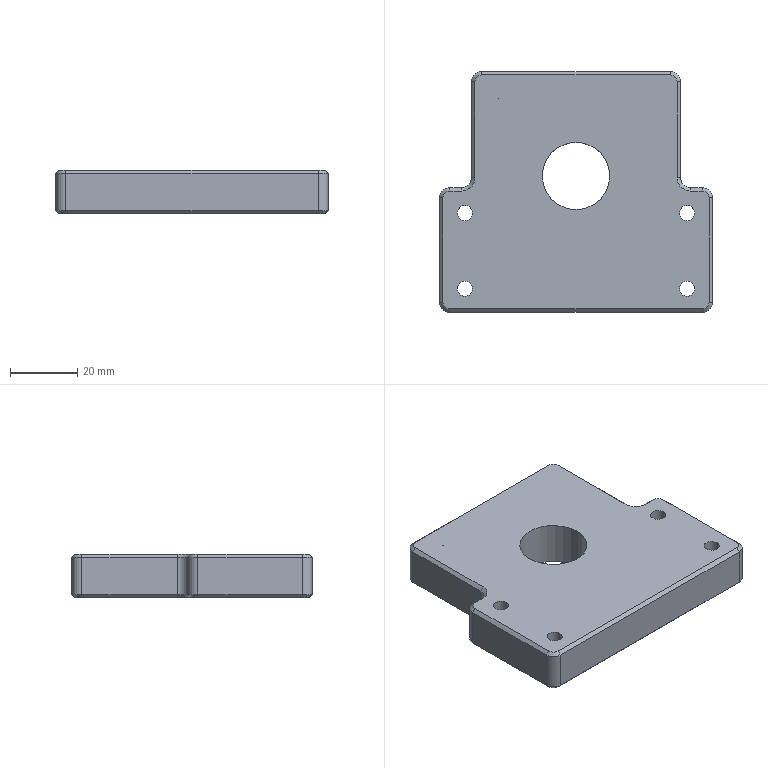Part | NX | features BREP 1 | 1 solid | 76 faces | box 81 x 71.5 x 13 mm | volume 60726 mm3 | plane 30 | cylinder 28 | cone 18 | commonest cylinder face diameters 4.5 x8 6 x8 8 x8 3.3 x2 20 x2